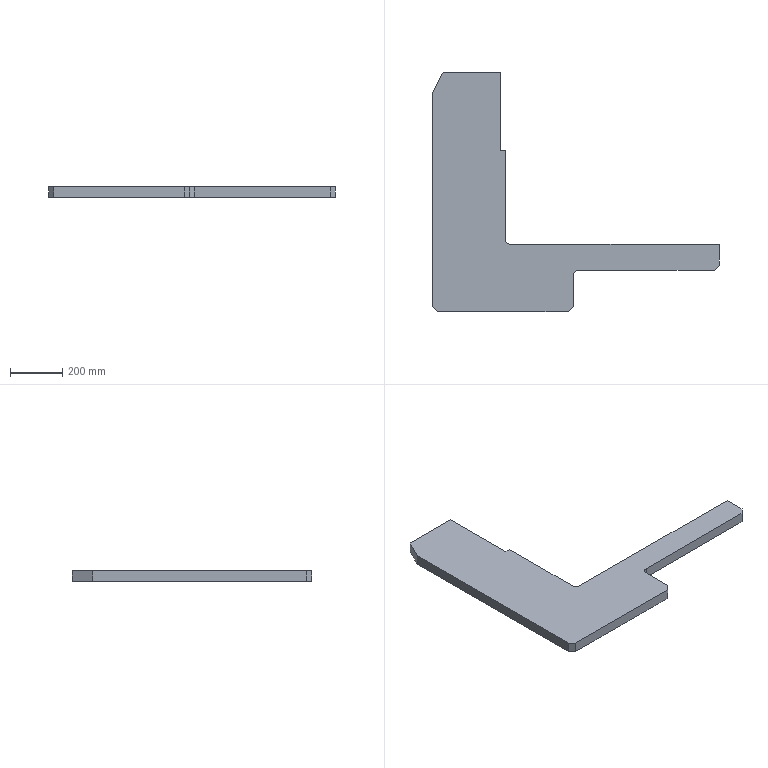Part | SolidWorks | features Chamfer 1, Extrusion 1, Fillet 1 | 1 solid | 18 faces | box 1099 x 919 x 40 mm | volume 14868507 mm3 | plane 16 | cylinder 2 | commonest cylinder face diameters 40 x2
STEP:
#1=CARTESIAN_POINT('',(-552.579,-80.753,0.));
#2=VERTEX_POINT('',#1);
#3=CARTESIAN_POINT('',(-53.579,-80.753,0.));
#4=VERTEX_POINT('',#3);
#5=CARTESIAN_POINT('',(-572.579,-80.753,0.));
#6=DIRECTION('',(1.,0.,0.));
#7=VECTOR('',#6,1000.);
#8=LINE('',#5,#7);
#9=EDGE_CURVE('',#2,#4,#8,.T.);
#10=ORIENTED_EDGE('',*,*,#9,.T.);
#11=CARTESIAN_POINT('',(-53.579,-80.753,40.));
#12=VERTEX_POINT('',#11);
#13=CARTESIAN_POINT('',(-53.579,-80.753,40.));
#14=DIRECTION('',(0.,0.,1.));
#15=VECTOR('',#14,1000.);
#16=LINE('',#13,#15);
#17=EDGE_CURVE('',#4,#12,#16,.T.);
#18=ORIENTED_EDGE('',*,*,#17,.T.);
#19=CARTESIAN_POINT('',(-552.579,-80.753,40.));
#20=VERTEX_POINT('',#19);
#21=CARTESIAN_POINT('',(-572.579,-80.753,40.));
#22=DIRECTION('',(1.,0.,0.));
#23=VECTOR('',#22,1000.);
#24=LINE('',#21,#23);
#25=EDGE_CURVE('',#20,#12,#24,.T.);
#26=ORIENTED_EDGE('',*,*,#25,.F.);
#27=CARTESIAN_POINT('',(-552.579,-80.753,40.));
#28=DIRECTION('',(0.,0.,-1.));
#29=VECTOR('',#28,1000.);
#30=LINE('',#27,#29);
#31=EDGE_CURVE('',#20,#2,#30,.T.);
#32=ORIENTED_EDGE('',*,*,#31,.T.);
#33=EDGE_LOOP('',(#10,#18,#26,#32));
#34=FACE_OUTER_BOUND('',#33,.T.);
#35=CARTESIAN_POINT('',(-572.579,-80.753,40.));
#36=DIRECTION('',(0.,1.,0.));
#37=DIRECTION('',(0.,0.,1.));
#38=AXIS2_PLACEMENT_3D('',#35,#36,#37);
#39=PLANE('',#38);
#40=ADVANCED_FACE('',(#34),#39,.F.);
#41=CARTESIAN_POINT('',(-33.579,-60.753,0.));
#42=VERTEX_POINT('',#41);
#43=CARTESIAN_POINT('',(-33.579,58.247,0.));
#44=VERTEX_POINT('',#43);
#45=CARTESIAN_POINT('',(-33.579,-80.753,0.));
#46=DIRECTION('',(0.,1.,0.));
#47=VECTOR('',#46,1000.);
#48=LINE('',#45,#47);
#49=EDGE_CURVE('',#42,#44,#48,.T.);
#50=ORIENTED_EDGE('',*,*,#49,.T.);
#51=CARTESIAN_POINT('',(-33.579,58.247,40.));
#52=VERTEX_POINT('',#51);
#53=CARTESIAN_POINT('',(-33.579,58.247,40.));
#54=DIRECTION('',(0.,0.,1.));
#55=VECTOR('',#54,1000.);
#56=LINE('',#53,#55);
#57=EDGE_CURVE('',#44,#52,#56,.T.);
#58=ORIENTED_EDGE('',*,*,#57,.T.);
#59=CARTESIAN_POINT('',(-33.579,-60.753,40.));
#60=VERTEX_POINT('',#59);
#61=CARTESIAN_POINT('',(-33.579,-80.753,40.));
#62=DIRECTION('',(0.,1.,0.));
#63=VECTOR('',#62,1000.);
#64=LINE('',#61,#63);
#65=EDGE_CURVE('',#60,#52,#64,.T.);
#66=ORIENTED_EDGE('',*,*,#65,.F.);
#67=CARTESIAN_POINT('',(-33.579,-60.753,40.));
#68=DIRECTION('',(0.,0.,-1.));
#69=VECTOR('',#68,1000.);
#70=LINE('',#67,#69);
#71=EDGE_CURVE('',#60,#42,#70,.T.);
#72=ORIENTED_EDGE('',*,*,#71,.T.);
#73=EDGE_LOOP('',(#50,#58,#66,#72));
#74=FACE_OUTER_BOUND('',#73,.T.);
#75=CARTESIAN_POINT('',(-33.579,-80.753,40.));
#76=DIRECTION('',(-1.,0.,0.));
#77=DIRECTION('',(0.,0.,1.));
#78=AXIS2_PLACEMENT_3D('',#75,#76,#77);
#79=PLANE('',#78);
#80=ADVANCED_FACE('',(#74),#79,.F.);
#81=CARTESIAN_POINT('',(-13.579,78.247,40.));
#82=VERTEX_POINT('',#81);
#83=CARTESIAN_POINT('',(506.421,78.247,40.));
#84=VERTEX_POINT('',#83);
#85=CARTESIAN_POINT('',(-33.579,78.247,40.));
#86=DIRECTION('',(1.,0.,0.));
#87=VECTOR('',#86,1000.);
#88=LINE('',#85,#87);
#89=EDGE_CURVE('',#82,#84,#88,.T.);
#90=ORIENTED_EDGE('',*,*,#89,.F.);
#91=CARTESIAN_POINT('',(-13.579,78.247,0.));
#92=VERTEX_POINT('',#91);
#93=CARTESIAN_POINT('',(-13.579,78.247,0.));
#94=DIRECTION('',(0.,0.,-1.));
#95=VECTOR('',#94,1000.);
#96=LINE('',#93,#95);
#97=EDGE_CURVE('',#82,#92,#96,.T.);
#98=ORIENTED_EDGE('',*,*,#97,.T.);
#99=CARTESIAN_POINT('',(506.421,78.247,0.));
#100=VERTEX_POINT('',#99);
#101=CARTESIAN_POINT('',(-33.579,78.247,0.));
#102=DIRECTION('',(1.,0.,0.));
#103=VECTOR('',#102,1000.);
#104=LINE('',#101,#103);
#105=EDGE_CURVE('',#92,#100,#104,.T.);
#106=ORIENTED_EDGE('',*,*,#105,.T.);
#107=CARTESIAN_POINT('',(506.421,78.247,40.));
#108=DIRECTION('',(0.,0.,1.));
#109=VECTOR('',#108,1000.);
#110=LINE('',#107,#109);
#111=EDGE_CURVE('',#100,#84,#110,.T.);
#112=ORIENTED_EDGE('',*,*,#111,.T.);
#113=EDGE_LOOP('',(#90,#98,#106,#112));
#114=FACE_OUTER_BOUND('',#113,.T.);
#115=CARTESIAN_POINT('',(-33.579,78.247,40.));
#116=DIRECTION('',(0.,1.,0.));
#117=DIRECTION('',(0.,0.,1.));
#118=AXIS2_PLACEMENT_3D('',#115,#116,#117);
#119=PLANE('',#118);
#120=ADVANCED_FACE('',(#114),#119,.F.);
#121=CARTESIAN_POINT('',(526.421,98.247,40.));
#122=VERTEX_POINT('',#121);
#123=CARTESIAN_POINT('',(526.421,178.247,40.));
#124=VERTEX_POINT('',#123);
#125=CARTESIAN_POINT('',(526.421,78.247,40.));
#126=DIRECTION('',(0.,1.,0.));
#127=VECTOR('',#126,1000.);
#128=LINE('',#125,#127);
#129=EDGE_CURVE('',#122,#124,#128,.T.);
#130=ORIENTED_EDGE('',*,*,#129,.F.);
#131=CARTESIAN_POINT('',(526.421,98.247,0.));
#132=VERTEX_POINT('',#131);
#133=CARTESIAN_POINT('',(526.421,98.247,40.));
#134=DIRECTION('',(0.,0.,-1.));
#135=VECTOR('',#134,1000.);
#136=LINE('',#133,#135);
#137=EDGE_CURVE('',#122,#132,#136,.T.);
#138=ORIENTED_EDGE('',*,*,#137,.T.);
#139=CARTESIAN_POINT('',(526.421,178.247,0.));
#140=VERTEX_POINT('',#139);
#141=CARTESIAN_POINT('',(526.421,78.247,0.));
#142=DIRECTION('',(0.,1.,0.));
#143=VECTOR('',#142,1000.);
#144=LINE('',#141,#143);
#145=EDGE_CURVE('',#132,#140,#144,.T.);
#146=ORIENTED_EDGE('',*,*,#145,.T.);
#147=CARTESIAN_POINT('',(526.421,178.247,40.));
#148=DIRECTION('',(0.,0.,-1.));
#149=VECTOR('',#148,1000.);
#150=LINE('',#147,#149);
#151=EDGE_CURVE('',#124,#140,#150,.T.);
#152=ORIENTED_EDGE('',*,*,#151,.F.);
#153=EDGE_LOOP('',(#130,#138,#146,#152));
#154=FACE_OUTER_BOUND('',#153,.T.);
#155=CARTESIAN_POINT('',(526.421,78.247,40.));
#156=DIRECTION('',(-1.,0.,0.));
#157=DIRECTION('',(0.,0.,1.));
#158=AXIS2_PLACEMENT_3D('',#155,#156,#157);
#159=PLANE('',#158);
#160=ADVANCED_FACE('',(#154),#159,.F.);
#161=CARTESIAN_POINT('',(-273.579,178.247,0.));
#162=VERTEX_POINT('',#161);
#163=CARTESIAN_POINT('',(526.421,178.247,0.));
#164=DIRECTION('',(-1.,0.,0.));
#165=VECTOR('',#164,1000.);
#166=LINE('',#163,#165);
#167=EDGE_CURVE('',#140,#162,#166,.T.);
#168=ORIENTED_EDGE('',*,*,#167,.T.);
#169=CARTESIAN_POINT('',(-273.579,178.247,40.));
#170=VERTEX_POINT('',#169);
#171=CARTESIAN_POINT('',(-273.579,178.247,40.));
#172=DIRECTION('',(0.,0.,1.));
#173=VECTOR('',#172,1000.);
#174=LINE('',#171,#173);
#175=EDGE_CURVE('',#162,#170,#174,.T.);
#176=ORIENTED_EDGE('',*,*,#175,.T.);
#177=CARTESIAN_POINT('',(526.421,178.247,40.));
#178=DIRECTION('',(-1.,0.,0.));
#179=VECTOR('',#178,1000.);
#180=LINE('',#177,#179);
#181=EDGE_CURVE('',#124,#170,#180,.T.);
#182=ORIENTED_EDGE('',*,*,#181,.F.);
#183=ORIENTED_EDGE('',*,*,#151,.T.);
#184=EDGE_LOOP('',(#168,#176,#182,#183));
#185=FACE_OUTER_BOUND('',#184,.T.);
#186=CARTESIAN_POINT('',(526.421,178.247,40.));
#187=DIRECTION('',(0.,-1.,0.));
#188=DIRECTION('',(1.,0.,0.));
#189=AXIS2_PLACEMENT_3D('',#186,#187,#188);
#190=PLANE('',#189);
#191=ADVANCED_FACE('',(#185),#190,.F.);
#192=CARTESIAN_POINT('',(-293.579,198.247,40.));
#193=VERTEX_POINT('',#192);
#194=CARTESIAN_POINT('',(-293.579,538.247,40.));
#195=VERTEX_POINT('',#194);
#196=CARTESIAN_POINT('',(-293.579,178.247,40.));
#197=DIRECTION('',(0.,1.,0.));
#198=VECTOR('',#197,1000.);
#199=LINE('',#196,#198);
#200=EDGE_CURVE('',#193,#195,#199,.T.);
#201=ORIENTED_EDGE('',*,*,#200,.F.);
#202=CARTESIAN_POINT('',(-293.579,198.247,0.));
#203=VERTEX_POINT('',#202);
#204=CARTESIAN_POINT('',(-293.579,198.247,0.));
#205=DIRECTION('',(0.,0.,-1.));
#206=VECTOR('',#205,1000.);
#207=LINE('',#204,#206);
#208=EDGE_CURVE('',#193,#203,#207,.T.);
#209=ORIENTED_EDGE('',*,*,#208,.T.);
#210=CARTESIAN_POINT('',(-293.579,538.247,0.));
#211=VERTEX_POINT('',#210);
#212=CARTESIAN_POINT('',(-293.579,178.247,0.));
#213=DIRECTION('',(0.,1.,0.));
#214=VECTOR('',#213,1000.);
#215=LINE('',#212,#214);
#216=EDGE_CURVE('',#203,#211,#215,.T.);
#217=ORIENTED_EDGE('',*,*,#216,.T.);
#218=CARTESIAN_POINT('',(-293.579,538.247,40.));
#219=DIRECTION('',(0.,0.,-1.));
#220=VECTOR('',#219,1000.);
#221=LINE('',#218,#220);
#222=EDGE_CURVE('',#195,#211,#221,.T.);
#223=ORIENTED_EDGE('',*,*,#222,.F.);
#224=EDGE_LOOP('',(#201,#209,#217,#223));
#225=FACE_OUTER_BOUND('',#224,.T.);
#226=CARTESIAN_POINT('',(-293.579,178.247,40.));
#227=DIRECTION('',(-1.,0.,0.));
#228=DIRECTION('',(0.,0.,1.));
#229=AXIS2_PLACEMENT_3D('',#226,#227,#228);
#230=PLANE('',#229);
#231=ADVANCED_FACE('',(#225),#230,.F.);
#232=CARTESIAN_POINT('',(-313.579,538.247,0.));
#233=VERTEX_POINT('',#232);
#234=CARTESIAN_POINT('',(-293.579,538.247,0.));
#235=DIRECTION('',(-1.,0.,0.));
#236=VECTOR('',#235,1000.);
#237=LINE('',#234,#236);
#238=EDGE_CURVE('',#211,#233,#237,.T.);
#239=ORIENTED_EDGE('',*,*,#238,.T.);
#240=CARTESIAN_POINT('',(-313.579,538.247,40.));
#241=VERTEX_POINT('',#240);
#242=CARTESIAN_POINT('',(-313.579,538.247,40.));
#243=DIRECTION('',(0.,0.,-1.));
#244=VECTOR('',#243,1000.);
#245=LINE('',#242,#244);
#246=EDGE_CURVE('',#241,#233,#245,.T.);
#247=ORIENTED_EDGE('',*,*,#246,.F.);
#248=CARTESIAN_POINT('',(-293.579,538.247,40.));
#249=DIRECTION('',(-1.,0.,0.));
#250=VECTOR('',#249,1000.);
#251=LINE('',#248,#250);
#252=EDGE_CURVE('',#195,#241,#251,.T.);
#253=ORIENTED_EDGE('',*,*,#252,.F.);
#254=ORIENTED_EDGE('',*,*,#222,.T.);
#255=EDGE_LOOP('',(#239,#247,#253,#254));
#256=FACE_OUTER_BOUND('',#255,.T.);
#257=CARTESIAN_POINT('',(-293.579,538.247,40.));
#258=DIRECTION('',(0.,-1.,0.));
#259=DIRECTION('',(0.,0.,-1.));
#260=AXIS2_PLACEMENT_3D('',#257,#258,#259);
#261=PLANE('',#260);
#262=ADVANCED_FACE('',(#256),#261,.F.);
#263=CARTESIAN_POINT('',(-313.579,838.247,0.));
#264=VERTEX_POINT('',#263);
#265=CARTESIAN_POINT('',(-313.579,538.247,0.));
#266=DIRECTION('',(0.,1.,0.));
#267=VECTOR('',#266,1000.);
#268=LINE('',#265,#267);
#269=EDGE_CURVE('',#233,#264,#268,.T.);
#270=ORIENTED_EDGE('',*,*,#269,.T.);
#271=CARTESIAN_POINT('',(-313.579,838.247,40.));
#272=VERTEX_POINT('',#271);
#273=CARTESIAN_POINT('',(-313.579,838.247,40.));
#274=DIRECTION('',(0.,0.,-1.));
#275=VECTOR('',#274,1000.);
#276=LINE('',#273,#275);
#277=EDGE_CURVE('',#272,#264,#276,.T.);
#278=ORIENTED_EDGE('',*,*,#277,.F.);
#279=CARTESIAN_POINT('',(-313.579,538.247,40.));
#280=DIRECTION('',(0.,1.,0.));
#281=VECTOR('',#280,1000.);
#282=LINE('',#279,#281);
#283=EDGE_CURVE('',#241,#272,#282,.T.);
#284=ORIENTED_EDGE('',*,*,#283,.F.);
#285=ORIENTED_EDGE('',*,*,#246,.T.);
#286=EDGE_LOOP('',(#270,#278,#284,#285));
#287=FACE_OUTER_BOUND('',#286,.T.);
#288=CARTESIAN_POINT('',(-313.579,538.247,40.));
#289=DIRECTION('',(-1.,0.,0.));
#290=DIRECTION('',(0.,0.,1.));
#291=AXIS2_PLACEMENT_3D('',#288,#289,#290);
#292=PLANE('',#291);
#293=ADVANCED_FACE('',(#287),#292,.F.);
#294=CARTESIAN_POINT('',(-532.579,838.247,0.));
#295=VERTEX_POINT('',#294);
#296=CARTESIAN_POINT('',(-313.579,838.247,0.));
#297=DIRECTION('',(-1.,0.,0.));
#298=VECTOR('',#297,1000.);
#299=LINE('',#296,#298);
#300=EDGE_CURVE('',#264,#295,#299,.T.);
#301=ORIENTED_EDGE('',*,*,#300,.T.);
#302=CARTESIAN_POINT('',(-532.579,838.247,40.));
#303=VERTEX_POINT('',#302);
#304=CARTESIAN_POINT('',(-532.579,838.247,40.));
#305=DIRECTION('',(0.,0.,-1.));
#306=VECTOR('',#305,1000.);
#307=LINE('',#304,#306);
#308=EDGE_CURVE('',#303,#295,#307,.T.);
#309=ORIENTED_EDGE('',*,*,#308,.F.);
#310=CARTESIAN_POINT('',(-313.579,838.247,40.));
#311=DIRECTION('',(-1.,0.,0.));
#312=VECTOR('',#311,1000.);
#313=LINE('',#310,#312);
#314=EDGE_CURVE('',#272,#303,#313,.T.);
#315=ORIENTED_EDGE('',*,*,#314,.F.);
#316=ORIENTED_EDGE('',*,*,#277,.T.);
#317=EDGE_LOOP('',(#301,#309,#315,#316));
#318=FACE_OUTER_BOUND('',#317,.T.);
#319=CARTESIAN_POINT('',(-313.579,838.247,40.));
#320=DIRECTION('',(0.,-1.,0.));
#321=DIRECTION('',(0.,0.,-1.));
#322=AXIS2_PLACEMENT_3D('',#319,#320,#321);
#323=PLANE('',#322);
#324=ADVANCED_FACE('',(#318),#323,.F.);
#325=CARTESIAN_POINT('',(-572.579,758.247,0.));
#326=VERTEX_POINT('',#325);
#327=CARTESIAN_POINT('',(-572.579,758.247,0.));
#328=DIRECTION('',(-0.4472,-0.8944,0.));
#329=VECTOR('',#328,1000.);
#330=LINE('',#327,#329);
#331=EDGE_CURVE('',#295,#326,#330,.T.);
#332=ORIENTED_EDGE('',*,*,#331,.T.);
#333=CARTESIAN_POINT('',(-572.579,758.247,40.));
#334=VERTEX_POINT('',#333);
#335=CARTESIAN_POINT('',(-572.579,758.247,40.));
#336=DIRECTION('',(0.,0.,-1.));
#337=VECTOR('',#336,1000.);
#338=LINE('',#335,#337);
#339=EDGE_CURVE('',#334,#326,#338,.T.);
#340=ORIENTED_EDGE('',*,*,#339,.F.);
#341=CARTESIAN_POINT('',(-572.579,758.247,40.));
#342=DIRECTION('',(-0.4472,-0.8944,0.));
#343=VECTOR('',#342,1000.);
#344=LINE('',#341,#343);
#345=EDGE_CURVE('',#303,#334,#344,.T.);
#346=ORIENTED_EDGE('',*,*,#345,.F.);
#347=ORIENTED_EDGE('',*,*,#308,.T.);
#348=EDGE_LOOP('',(#332,#340,#346,#347));
#349=FACE_OUTER_BOUND('',#348,.T.);
#350=CARTESIAN_POINT('',(-572.579,758.247,40.));
#351=DIRECTION('',(0.8944,-0.4472,0.));
#352=DIRECTION('',(0.4472,0.8944,0.));
#353=AXIS2_PLACEMENT_3D('',#350,#351,#352);
#354=PLANE('',#353);
#355=ADVANCED_FACE('',(#349),#354,.F.);
#356=CARTESIAN_POINT('',(-572.579,-60.753,0.));
#357=VERTEX_POINT('',#356);
#358=CARTESIAN_POINT('',(-572.579,758.247,0.));
#359=DIRECTION('',(0.,-1.,0.));
#360=VECTOR('',#359,1000.);
#361=LINE('',#358,#360);
#362=EDGE_CURVE('',#326,#357,#361,.T.);
#363=ORIENTED_EDGE('',*,*,#362,.T.);
#364=CARTESIAN_POINT('',(-572.579,-60.753,40.));
#365=VERTEX_POINT('',#364);
#366=CARTESIAN_POINT('',(-572.579,-60.753,40.));
#367=DIRECTION('',(0.,0.,1.));
#368=VECTOR('',#367,1000.);
#369=LINE('',#366,#368);
#370=EDGE_CURVE('',#357,#365,#369,.T.);
#371=ORIENTED_EDGE('',*,*,#370,.T.);
#372=CARTESIAN_POINT('',(-572.579,758.247,40.));
#373=DIRECTION('',(0.,-1.,0.));
#374=VECTOR('',#373,1000.);
#375=LINE('',#372,#374);
#376=EDGE_CURVE('',#334,#365,#375,.T.);
#377=ORIENTED_EDGE('',*,*,#376,.F.);
#378=ORIENTED_EDGE('',*,*,#339,.T.);
#379=EDGE_LOOP('',(#363,#371,#377,#378));
#380=FACE_OUTER_BOUND('',#379,.T.);
#381=CARTESIAN_POINT('',(-572.579,758.247,40.));
#382=DIRECTION('',(1.,0.,0.));
#383=DIRECTION('',(0.,1.,0.));
#384=AXIS2_PLACEMENT_3D('',#381,#382,#383);
#385=PLANE('',#384);
#386=ADVANCED_FACE('',(#380),#385,.F.);
#387=ORIENTED_EDGE('',*,*,#65,.T.);
#388=CARTESIAN_POINT('',(-13.579,58.247,40.));
#389=DIRECTION('',(0.,0.,-1.));
#390=DIRECTION('',(1.,0.,0.));
#391=AXIS2_PLACEMENT_3D('',#388,#389,#390);
#392=CIRCLE('',#391,20.);
#393=EDGE_CURVE('',#52,#82,#392,.T.);
#394=ORIENTED_EDGE('',*,*,#393,.T.);
#395=ORIENTED_EDGE('',*,*,#89,.T.);
#396=CARTESIAN_POINT('',(214.087,-214.087,40.));
#397=DIRECTION('',(0.7071,0.7071,0.));
#398=VECTOR('',#397,1000.);
#399=LINE('',#396,#398);
#400=EDGE_CURVE('',#84,#122,#399,.T.);
#401=ORIENTED_EDGE('',*,*,#400,.T.);
#402=ORIENTED_EDGE('',*,*,#129,.T.);
#403=ORIENTED_EDGE('',*,*,#181,.T.);
#404=CARTESIAN_POINT('',(-273.579,198.247,40.));
#405=DIRECTION('',(0.,0.,-1.));
#406=DIRECTION('',(1.,0.,0.));
#407=AXIS2_PLACEMENT_3D('',#404,#405,#406);
#408=CIRCLE('',#407,20.);
#409=EDGE_CURVE('',#170,#193,#408,.T.);
#410=ORIENTED_EDGE('',*,*,#409,.T.);
#411=ORIENTED_EDGE('',*,*,#200,.T.);
#412=ORIENTED_EDGE('',*,*,#252,.T.);
#413=ORIENTED_EDGE('',*,*,#283,.T.);
#414=ORIENTED_EDGE('',*,*,#314,.T.);
#415=ORIENTED_EDGE('',*,*,#345,.T.);
#416=ORIENTED_EDGE('',*,*,#376,.T.);
#417=CARTESIAN_POINT('',(-316.666,-316.666,40.));
#418=DIRECTION('',(0.7071,-0.7071,0.));
#419=VECTOR('',#418,1000.);
#420=LINE('',#417,#419);
#421=EDGE_CURVE('',#365,#20,#420,.T.);
#422=ORIENTED_EDGE('',*,*,#421,.T.);
#423=ORIENTED_EDGE('',*,*,#25,.T.);
#424=CARTESIAN_POINT('',(13.587,-13.587,40.));
#425=DIRECTION('',(0.7071,0.7071,0.));
#426=VECTOR('',#425,1000.);
#427=LINE('',#424,#426);
#428=EDGE_CURVE('',#12,#60,#427,.T.);
#429=ORIENTED_EDGE('',*,*,#428,.T.);
#430=EDGE_LOOP('',(#387,#394,#395,#401,#402,#403,#410,#411,#412,#413,#414,#415,#416,#422,#423,#429));
#431=FACE_OUTER_BOUND('',#430,.T.);
#432=CARTESIAN_POINT('',(0.,0.,40.));
#433=DIRECTION('',(0.,0.,1.));
#434=DIRECTION('',(1.,0.,0.));
#435=AXIS2_PLACEMENT_3D('',#432,#433,#434);
#436=PLANE('',#435);
#437=ADVANCED_FACE('',(#431),#436,.T.);
#438=ORIENTED_EDGE('',*,*,#145,.F.);
#439=CARTESIAN_POINT('',(526.421,98.247,0.));
#440=DIRECTION('',(-0.7071,-0.7071,0.));
#441=VECTOR('',#440,1000.);
#442=LINE('',#439,#441);
#443=EDGE_CURVE('',#132,#100,#442,.T.);
#444=ORIENTED_EDGE('',*,*,#443,.T.);
#445=ORIENTED_EDGE('',*,*,#105,.F.);
#446=CARTESIAN_POINT('',(-13.579,58.247,0.));
#447=DIRECTION('',(0.,0.,1.));
#448=DIRECTION('',(1.,0.,0.));
#449=AXIS2_PLACEMENT_3D('',#446,#447,#448);
#450=CIRCLE('',#449,20.);
#451=EDGE_CURVE('',#92,#44,#450,.T.);
#452=ORIENTED_EDGE('',*,*,#451,.T.);
#453=ORIENTED_EDGE('',*,*,#49,.F.);
#454=CARTESIAN_POINT('',(-33.579,-60.753,0.));
#455=DIRECTION('',(-0.7071,-0.7071,0.));
#456=VECTOR('',#455,1000.);
#457=LINE('',#454,#456);
#458=EDGE_CURVE('',#42,#4,#457,.T.);
#459=ORIENTED_EDGE('',*,*,#458,.T.);
#460=ORIENTED_EDGE('',*,*,#9,.F.);
#461=CARTESIAN_POINT('',(-552.579,-80.753,0.));
#462=DIRECTION('',(-0.7071,0.7071,0.));
#463=VECTOR('',#462,1000.);
#464=LINE('',#461,#463);
#465=EDGE_CURVE('',#2,#357,#464,.T.);
#466=ORIENTED_EDGE('',*,*,#465,.T.);
#467=ORIENTED_EDGE('',*,*,#362,.F.);
#468=ORIENTED_EDGE('',*,*,#331,.F.);
#469=ORIENTED_EDGE('',*,*,#300,.F.);
#470=ORIENTED_EDGE('',*,*,#269,.F.);
#471=ORIENTED_EDGE('',*,*,#238,.F.);
#472=ORIENTED_EDGE('',*,*,#216,.F.);
#473=CARTESIAN_POINT('',(-273.579,198.247,0.));
#474=DIRECTION('',(0.,0.,1.));
#475=DIRECTION('',(1.,0.,0.));
#476=AXIS2_PLACEMENT_3D('',#473,#474,#475);
#477=CIRCLE('',#476,20.);
#478=EDGE_CURVE('',#203,#162,#477,.T.);
#479=ORIENTED_EDGE('',*,*,#478,.T.);
#480=ORIENTED_EDGE('',*,*,#167,.F.);
#481=EDGE_LOOP('',(#438,#444,#445,#452,#453,#459,#460,#466,#467,#468,#469,#470,#471,#472,#479,#480));
#482=FACE_OUTER_BOUND('',#481,.T.);
#483=CARTESIAN_POINT('',(0.,0.,0.));
#484=DIRECTION('',(0.,0.,1.));
#485=DIRECTION('',(1.,0.,0.));
#486=AXIS2_PLACEMENT_3D('',#483,#484,#485);
#487=PLANE('',#486);
#488=ADVANCED_FACE('',(#482),#487,.F.);
#489=ORIENTED_EDGE('',*,*,#400,.F.);
#490=ORIENTED_EDGE('',*,*,#111,.F.);
#491=ORIENTED_EDGE('',*,*,#443,.F.);
#492=ORIENTED_EDGE('',*,*,#137,.F.);
#493=EDGE_LOOP('',(#489,#490,#491,#492));
#494=FACE_OUTER_BOUND('',#493,.T.);
#495=CARTESIAN_POINT('',(526.421,98.247,40.));
#496=DIRECTION('',(-0.7071,0.7071,0.));
#497=DIRECTION('',(0.,0.,-1.));
#498=AXIS2_PLACEMENT_3D('',#495,#496,#497);
#499=PLANE('',#498);
#500=ADVANCED_FACE('',(#494),#499,.F.);
#501=ORIENTED_EDGE('',*,*,#428,.F.);
#502=ORIENTED_EDGE('',*,*,#17,.F.);
#503=ORIENTED_EDGE('',*,*,#458,.F.);
#504=ORIENTED_EDGE('',*,*,#71,.F.);
#505=EDGE_LOOP('',(#501,#502,#503,#504));
#506=FACE_OUTER_BOUND('',#505,.T.);
#507=CARTESIAN_POINT('',(-33.579,-60.753,40.));
#508=DIRECTION('',(-0.7071,0.7071,0.));
#509=DIRECTION('',(0.,0.,-1.));
#510=AXIS2_PLACEMENT_3D('',#507,#508,#509);
#511=PLANE('',#510);
#512=ADVANCED_FACE('',(#506),#511,.F.);
#513=ORIENTED_EDGE('',*,*,#421,.F.);
#514=ORIENTED_EDGE('',*,*,#370,.F.);
#515=ORIENTED_EDGE('',*,*,#465,.F.);
#516=ORIENTED_EDGE('',*,*,#31,.F.);
#517=EDGE_LOOP('',(#513,#514,#515,#516));
#518=FACE_OUTER_BOUND('',#517,.T.);
#519=CARTESIAN_POINT('',(-552.579,-80.753,40.));
#520=DIRECTION('',(0.7071,0.7071,0.));
#521=DIRECTION('',(0.,0.,-1.));
#522=AXIS2_PLACEMENT_3D('',#519,#520,#521);
#523=PLANE('',#522);
#524=ADVANCED_FACE('',(#518),#523,.F.);
#525=ORIENTED_EDGE('',*,*,#393,.F.);
#526=ORIENTED_EDGE('',*,*,#57,.F.);
#527=ORIENTED_EDGE('',*,*,#451,.F.);
#528=ORIENTED_EDGE('',*,*,#97,.F.);
#529=EDGE_LOOP('',(#525,#526,#527,#528));
#530=FACE_OUTER_BOUND('',#529,.T.);
#531=CARTESIAN_POINT('',(-13.579,58.247,40.));
#532=DIRECTION('',(0.,0.,1.));
#533=DIRECTION('',(1.,0.,0.));
#534=AXIS2_PLACEMENT_3D('',#531,#532,#533);
#535=CYLINDRICAL_SURFACE('',#534,20.);
#536=ADVANCED_FACE('',(#530),#535,.F.);
#537=ORIENTED_EDGE('',*,*,#409,.F.);
#538=ORIENTED_EDGE('',*,*,#175,.F.);
#539=ORIENTED_EDGE('',*,*,#478,.F.);
#540=ORIENTED_EDGE('',*,*,#208,.F.);
#541=EDGE_LOOP('',(#537,#538,#539,#540));
#542=FACE_OUTER_BOUND('',#541,.T.);
#543=CARTESIAN_POINT('',(-273.579,198.247,40.));
#544=DIRECTION('',(0.,0.,1.));
#545=DIRECTION('',(1.,0.,0.));
#546=AXIS2_PLACEMENT_3D('',#543,#544,#545);
#547=CYLINDRICAL_SURFACE('',#546,20.);
#548=ADVANCED_FACE('',(#542),#547,.F.);
#549=CLOSED_SHELL('',(#40,#80,#120,#160,#191,#231,#262,#293,#324,#355,#386,#437,#488,#500,#512,#524,#536,#548));
#550=MANIFOLD_SOLID_BREP('',#549);
#551=CARTESIAN_POINT('',(0.,0.,0.));
#552=DIRECTION('',(0.,0.,1.));
#553=DIRECTION('',(1.,0.,0.));
#554=AXIS2_PLACEMENT_3D('',#551,#552,#553);
#555=(LENGTH_UNIT()NAMED_UNIT(*)SI_UNIT(.MILLI.,.METRE.));
#556=UNCERTAINTY_MEASURE_WITH_UNIT(LENGTH_MEASURE(0.00001),#555,'','');
#557=(NAMED_UNIT(*)PLANE_ANGLE_UNIT()SI_UNIT($,.RADIAN.));
#558=(NAMED_UNIT(*)SI_UNIT($,.STERADIAN.)SOLID_ANGLE_UNIT());
#559=(GEOMETRIC_REPRESENTATION_CONTEXT(3)GLOBAL_UNCERTAINTY_ASSIGNED_CONTEXT((#556))GLOBAL_UNIT_ASSIGNED_CONTEXT((#555,#557,#558))REPRESENTATION_CONTEXT('',''));
#560=ADVANCED_BREP_SHAPE_REPRESENTATION('',(#550,#554),#559);